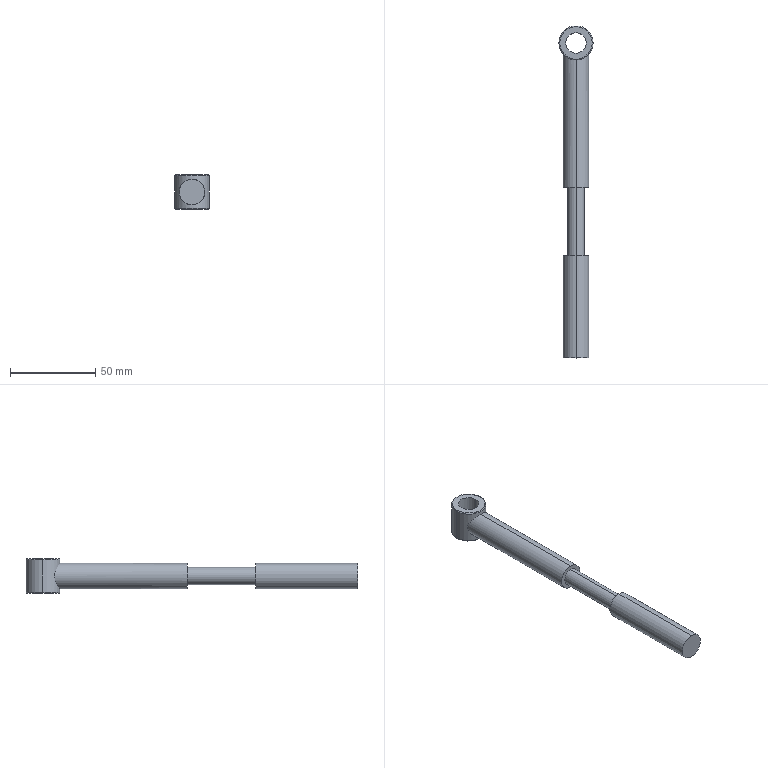Part | STEP file | piston rod | 1 solid | 19 faces | box 20 x 194.5 x 20 mm | volume 31059 mm3 | cylinder 10 | plane 5 | torus 4 | commonest cylinder face diameters 15 x4 10 x2 12 x2 20 x2
STEP:
#1=CARTESIAN_POINT('',(-10.,104.5,9.5));
#2=VERTEX_POINT('',#1);
#3=CARTESIAN_POINT('',(10.,104.5,9.5));
#4=VERTEX_POINT('',#3);
#5=CARTESIAN_POINT('',(0.,104.5,9.5));
#6=DIRECTION('',(0.,0.,-1.));
#7=DIRECTION('',(1.,0.,0.));
#8=AXIS2_PLACEMENT_3D('',#5,#6,#7);
#9=CIRCLE('',#8,10.);
#10=EDGE_CURVE('',#2,#4,#9,.T.);
#11=ORIENTED_EDGE('',*,*,#10,.F.);
#12=CARTESIAN_POINT('',(-9.5,104.5,10.));
#13=VERTEX_POINT('',#12);
#14=CARTESIAN_POINT('',(-9.5,104.5,9.5));
#15=DIRECTION('',(0.,1.,0.));
#16=DIRECTION('',(-1.,0.,0.));
#17=AXIS2_PLACEMENT_3D('',#14,#15,#16);
#18=CIRCLE('',#17,0.5);
#19=EDGE_CURVE('',#2,#13,#18,.T.);
#20=ORIENTED_EDGE('',*,*,#19,.T.);
#21=CARTESIAN_POINT('',(9.5,104.5,10.));
#22=VERTEX_POINT('',#21);
#23=CARTESIAN_POINT('',(0.,104.5,10.));
#24=DIRECTION('',(0.,0.,1.));
#25=DIRECTION('',(1.,0.,0.));
#26=AXIS2_PLACEMENT_3D('',#23,#24,#25);
#27=CIRCLE('',#26,9.5);
#28=EDGE_CURVE('',#22,#13,#27,.T.);
#29=ORIENTED_EDGE('',*,*,#28,.F.);
#30=CARTESIAN_POINT('',(9.5,104.5,9.5));
#31=DIRECTION('',(0.,-1.,0.));
#32=DIRECTION('',(0.,0.,-1.));
#33=AXIS2_PLACEMENT_3D('',#30,#31,#32);
#34=CIRCLE('',#33,0.5);
#35=EDGE_CURVE('',#4,#22,#34,.T.);
#36=ORIENTED_EDGE('',*,*,#35,.F.);
#37=EDGE_LOOP('',(#11,#20,#29,#36));
#38=FACE_OUTER_BOUND('',#37,.T.);
#39=CARTESIAN_POINT('',(0.,104.5,9.5));
#40=DIRECTION('',(0.,0.,1.));
#41=DIRECTION('',(1.,0.,0.));
#42=AXIS2_PLACEMENT_3D('',#39,#40,#41);
#43=TOROIDAL_SURFACE('',#42,9.5,0.5);
#44=ADVANCED_FACE('',(#38),#43,.T.);
#45=CARTESIAN_POINT('',(-9.5,104.5,-10.));
#46=VERTEX_POINT('',#45);
#47=CARTESIAN_POINT('',(9.5,104.5,-10.));
#48=VERTEX_POINT('',#47);
#49=CARTESIAN_POINT('',(0.,104.5,-10.));
#50=DIRECTION('',(0.,0.,-1.));
#51=DIRECTION('',(1.,0.,0.));
#52=AXIS2_PLACEMENT_3D('',#49,#50,#51);
#53=CIRCLE('',#52,9.5);
#54=EDGE_CURVE('',#46,#48,#53,.T.);
#55=ORIENTED_EDGE('',*,*,#54,.F.);
#56=CARTESIAN_POINT('',(-10.,104.5,-9.5));
#57=VERTEX_POINT('',#56);
#58=CARTESIAN_POINT('',(-9.5,104.5,-9.5));
#59=DIRECTION('',(0.,1.,0.));
#60=DIRECTION('',(-1.,0.,0.));
#61=AXIS2_PLACEMENT_3D('',#58,#59,#60);
#62=CIRCLE('',#61,0.5);
#63=EDGE_CURVE('',#46,#57,#62,.T.);
#64=ORIENTED_EDGE('',*,*,#63,.T.);
#65=CARTESIAN_POINT('',(10.,104.5,-9.5));
#66=VERTEX_POINT('',#65);
#67=CARTESIAN_POINT('',(0.,104.5,-9.5));
#68=DIRECTION('',(0.,0.,1.));
#69=DIRECTION('',(1.,0.,0.));
#70=AXIS2_PLACEMENT_3D('',#67,#68,#69);
#71=CIRCLE('',#70,10.);
#72=EDGE_CURVE('',#66,#57,#71,.T.);
#73=ORIENTED_EDGE('',*,*,#72,.F.);
#74=CARTESIAN_POINT('',(9.5,104.5,-9.5));
#75=DIRECTION('',(0.,-1.,0.));
#76=DIRECTION('',(0.,0.,-1.));
#77=AXIS2_PLACEMENT_3D('',#74,#75,#76);
#78=CIRCLE('',#77,0.5);
#79=EDGE_CURVE('',#48,#66,#78,.T.);
#80=ORIENTED_EDGE('',*,*,#79,.F.);
#81=EDGE_LOOP('',(#55,#64,#73,#80));
#82=FACE_OUTER_BOUND('',#81,.T.);
#83=CARTESIAN_POINT('',(0.,104.5,-9.5));
#84=DIRECTION('',(0.,0.,1.));
#85=DIRECTION('',(1.,0.,0.));
#86=AXIS2_PLACEMENT_3D('',#83,#84,#85);
#87=TOROIDAL_SURFACE('',#86,9.5,0.5);
#88=ADVANCED_FACE('',(#82),#87,.T.);
#89=CARTESIAN_POINT('',(-6.,104.5,-10.));
#90=VERTEX_POINT('',#89);
#91=CARTESIAN_POINT('',(6.,104.5,-10.));
#92=VERTEX_POINT('',#91);
#93=CARTESIAN_POINT('',(0.,104.5,-10.));
#94=DIRECTION('',(0.,0.,1.));
#95=DIRECTION('',(1.,0.,0.));
#96=AXIS2_PLACEMENT_3D('',#93,#94,#95);
#97=CIRCLE('',#96,6.);
#98=EDGE_CURVE('',#90,#92,#97,.T.);
#99=ORIENTED_EDGE('',*,*,#98,.F.);
#100=CARTESIAN_POINT('',(-6.,104.5,10.));
#101=VERTEX_POINT('',#100);
#102=CARTESIAN_POINT('',(-6.,104.5,-10.));
#103=DIRECTION('',(0.,0.,1.));
#104=VECTOR('',#103,1000.);
#105=LINE('',#102,#104);
#106=EDGE_CURVE('',#90,#101,#105,.T.);
#107=ORIENTED_EDGE('',*,*,#106,.T.);
#108=CARTESIAN_POINT('',(6.,104.5,10.));
#109=VERTEX_POINT('',#108);
#110=CARTESIAN_POINT('',(0.,104.5,10.));
#111=DIRECTION('',(0.,0.,1.));
#112=DIRECTION('',(1.,0.,0.));
#113=AXIS2_PLACEMENT_3D('',#110,#111,#112);
#114=CIRCLE('',#113,6.);
#115=EDGE_CURVE('',#101,#109,#114,.T.);
#116=ORIENTED_EDGE('',*,*,#115,.T.);
#117=CARTESIAN_POINT('',(6.,104.5,-10.));
#118=DIRECTION('',(0.,0.,1.));
#119=VECTOR('',#118,1000.);
#120=LINE('',#117,#119);
#121=EDGE_CURVE('',#92,#109,#120,.T.);
#122=ORIENTED_EDGE('',*,*,#121,.F.);
#123=EDGE_LOOP('',(#99,#107,#116,#122));
#124=FACE_OUTER_BOUND('',#123,.T.);
#125=CARTESIAN_POINT('',(0.,104.5,-10.));
#126=DIRECTION('',(0.,0.,1.));
#127=DIRECTION('',(1.,0.,0.));
#128=AXIS2_PLACEMENT_3D('',#125,#126,#127);
#129=CYLINDRICAL_SURFACE('',#128,6.);
#130=ADVANCED_FACE('',(#124),#129,.F.);
#131=ORIENTED_EDGE('',*,*,#10,.T.);
#132=CARTESIAN_POINT('',(10.,104.5,10.));
#133=DIRECTION('',(0.,0.,-1.));
#134=VECTOR('',#133,1000.);
#135=LINE('',#132,#134);
#136=EDGE_CURVE('',#4,#66,#135,.T.);
#137=ORIENTED_EDGE('',*,*,#136,.T.);
#138=ORIENTED_EDGE('',*,*,#72,.T.);
#139=CARTESIAN_POINT('',(-10.,104.5,10.));
#140=DIRECTION('',(0.,0.,-1.));
#141=VECTOR('',#140,1000.);
#142=LINE('',#139,#141);
#143=EDGE_CURVE('',#2,#57,#142,.T.);
#144=ORIENTED_EDGE('',*,*,#143,.F.);
#145=EDGE_LOOP('',(#131,#137,#138,#144));
#146=FACE_OUTER_BOUND('',#145,.T.);
#147=CARTESIAN_POINT('',(0.,104.5,10.));
#148=DIRECTION('',(0.,0.,-1.));
#149=DIRECTION('',(-1.,0.,0.));
#150=AXIS2_PLACEMENT_3D('',#147,#148,#149);
#151=CYLINDRICAL_SURFACE('',#150,10.);
#152=ADVANCED_FACE('',(#146),#151,.T.);
#153=CARTESIAN_POINT('',(0.,-20.,5.));
#154=VERTEX_POINT('',#153);
#155=CARTESIAN_POINT('',(0.,-20.,-5.));
#156=VERTEX_POINT('',#155);
#157=CARTESIAN_POINT('',(0.,-20.,0.));
#158=DIRECTION('',(0.,1.,0.));
#159=DIRECTION('',(0.,0.,1.));
#160=AXIS2_PLACEMENT_3D('',#157,#158,#159);
#161=CIRCLE('',#160,5.);
#162=EDGE_CURVE('',#154,#156,#161,.T.);
#163=ORIENTED_EDGE('',*,*,#162,.T.);
#164=CARTESIAN_POINT('',(0.,20.,-5.));
#165=VERTEX_POINT('',#164);
#166=CARTESIAN_POINT('',(0.,27.897,-5.));
#167=DIRECTION('',(0.,1.,0.));
#168=VECTOR('',#167,1000.);
#169=LINE('',#166,#168);
#170=EDGE_CURVE('',#156,#165,#169,.T.);
#171=ORIENTED_EDGE('',*,*,#170,.T.);
#172=CARTESIAN_POINT('',(0.,20.,5.));
#173=VERTEX_POINT('',#172);
#174=CARTESIAN_POINT('',(0.,20.,0.));
#175=DIRECTION('',(0.,1.,0.));
#176=DIRECTION('',(0.,0.,1.));
#177=AXIS2_PLACEMENT_3D('',#174,#175,#176);
#178=CIRCLE('',#177,5.);
#179=EDGE_CURVE('',#173,#165,#178,.T.);
#180=ORIENTED_EDGE('',*,*,#179,.F.);
#181=CARTESIAN_POINT('',(0.,27.897,5.));
#182=DIRECTION('',(0.,1.,0.));
#183=VECTOR('',#182,1000.);
#184=LINE('',#181,#183);
#185=EDGE_CURVE('',#154,#173,#184,.T.);
#186=ORIENTED_EDGE('',*,*,#185,.F.);
#187=EDGE_LOOP('',(#163,#171,#180,#186));
#188=FACE_OUTER_BOUND('',#187,.T.);
#189=CARTESIAN_POINT('',(0.,27.897,0.));
#190=DIRECTION('',(0.,1.,0.));
#191=DIRECTION('',(0.,0.,1.));
#192=AXIS2_PLACEMENT_3D('',#189,#190,#191);
#193=CYLINDRICAL_SURFACE('',#192,5.);
#194=ADVANCED_FACE('',(#188),#193,.T.);
#195=CARTESIAN_POINT('',(0.,20.,7.5));
#196=VERTEX_POINT('',#195);
#197=CARTESIAN_POINT('',(0.,20.,-7.5));
#198=VERTEX_POINT('',#197);
#199=CARTESIAN_POINT('',(0.,20.,0.));
#200=DIRECTION('',(0.,1.,0.));
#201=DIRECTION('',(0.,0.,1.));
#202=AXIS2_PLACEMENT_3D('',#199,#200,#201);
#203=CIRCLE('',#202,7.5);
#204=EDGE_CURVE('',#196,#198,#203,.T.);
#205=ORIENTED_EDGE('',*,*,#204,.T.);
#206=CARTESIAN_POINT('',(0.,94.5,-7.5));
#207=VERTEX_POINT('',#206);
#208=CARTESIAN_POINT('',(0.,63.204,-7.5));
#209=DIRECTION('',(0.,1.,0.));
#210=VECTOR('',#209,1000.);
#211=LINE('',#208,#210);
#212=EDGE_CURVE('',#198,#207,#211,.T.);
#213=ORIENTED_EDGE('',*,*,#212,.T.);
#214=CARTESIAN_POINT('',(0.,94.5,7.5));
#215=VERTEX_POINT('',#214);
#216=CARTESIAN_POINT('',(0.,94.5,-7.5));
#217=CARTESIAN_POINT('',(0.2563,94.5,-7.5));
#218=CARTESIAN_POINT('',(0.516,94.51,-7.487));
#219=CARTESIAN_POINT('',(1.029,94.55,-7.434));
#220=CARTESIAN_POINT('',(1.282,94.579,-7.394));
#221=CARTESIAN_POINT('',(1.778,94.656,-7.291));
#222=CARTESIAN_POINT('',(2.022,94.703,-7.227));
#223=CARTESIAN_POINT('',(2.502,94.815,-7.075));
#224=CARTESIAN_POINT('',(2.739,94.879,-6.986));
#225=CARTESIAN_POINT('',(3.422,95.092,-6.692));
#226=CARTESIAN_POINT('',(3.847,95.259,-6.457));
#227=CARTESIAN_POINT('',(4.643,95.632,-5.91));
#228=CARTESIAN_POINT('',(5.006,95.835,-5.604));
#229=CARTESIAN_POINT('',(5.501,96.147,-5.103));
#230=CARTESIAN_POINT('',(5.658,96.252,-4.929));
#231=CARTESIAN_POINT('',(5.955,96.465,-4.565));
#232=CARTESIAN_POINT('',(6.097,96.572,-4.375));
#233=CARTESIAN_POINT('',(6.489,96.884,-3.789));
#234=CARTESIAN_POINT('',(6.714,97.085,-3.376));
#235=CARTESIAN_POINT('',(6.995,97.353,-2.715));
#236=CARTESIAN_POINT('',(7.08,97.437,-2.487));
#237=CARTESIAN_POINT('',(7.228,97.589,-2.015));
#238=CARTESIAN_POINT('',(7.292,97.657,-1.772));
#239=CARTESIAN_POINT('',(7.394,97.767,-1.279));
#240=CARTESIAN_POINT('',(7.434,97.811,-1.029));
#241=CARTESIAN_POINT('',(7.486,97.87,-0.5188));
#242=CARTESIAN_POINT('',(7.5,97.886,-0.2571));
#243=CARTESIAN_POINT('',(7.5,97.886,0.2591));
#244=CARTESIAN_POINT('',(7.487,97.87,0.515));
#245=CARTESIAN_POINT('',(7.434,97.812,1.023));
#246=CARTESIAN_POINT('',(7.395,97.768,1.276));
#247=CARTESIAN_POINT('',(7.24,97.601,2.021));
#248=CARTESIAN_POINT('',(7.092,97.445,2.487));
#249=CARTESIAN_POINT('',(6.809,97.175,3.153));
#250=CARTESIAN_POINT('',(6.704,97.079,3.371));
#251=CARTESIAN_POINT('',(6.476,96.879,3.79));
#252=CARTESIAN_POINT('',(6.354,96.776,3.992));
#253=CARTESIAN_POINT('',(5.962,96.464,4.575));
#254=CARTESIAN_POINT('',(5.667,96.252,4.935));
#255=CARTESIAN_POINT('',(5.171,95.938,5.438));
#256=CARTESIAN_POINT('',(4.995,95.834,5.6));
#257=CARTESIAN_POINT('',(4.63,95.634,5.905));
#258=CARTESIAN_POINT('',(4.441,95.538,6.048));
#259=CARTESIAN_POINT('',(3.852,95.262,6.453));
#260=CARTESIAN_POINT('',(3.431,95.095,6.688));
#261=CARTESIAN_POINT('',(2.748,94.882,6.983));
#262=CARTESIAN_POINT('',(2.511,94.817,7.072));
#263=CARTESIAN_POINT('',(2.03,94.705,7.224));
#264=CARTESIAN_POINT('',(1.786,94.658,7.289));
#265=CARTESIAN_POINT('',(1.289,94.58,7.393));
#266=CARTESIAN_POINT('',(1.036,94.55,7.433));
#267=CARTESIAN_POINT('',(0.5214,94.51,7.486));
#268=CARTESIAN_POINT('',(0.2596,94.5,7.5));
#269=CARTESIAN_POINT('',(0.,94.5,7.5));
#270=B_SPLINE_CURVE_WITH_KNOTS('',3,(#216,#217,#218,#219,#220,#221,#222,#223,#224,#225,#226,#227,#228,#229,#230,#231,#232,#233,#234,#235,#236,#237,#238,#239,#240,#241,#242,#243,#244,#245,#246,#247,#248,#249,#250,#251,#252,#253,#254,#255,#256,#257,#258,#259,#260,#261,#262,#263,#264,#265,#266,#267,#268,#269),.UNSPECIFIED.,.F.,.F.,(4,2,2,2,2,2,2,2,2,2,2,2,2,2,2,2,2,2,2,2,2,2,2,2,2,2,4),(0.02456,0.02533,0.0261,0.02686,0.02763,0.02916,0.03069,0.03146,0.03222,0.03376,0.03452,0.03529,0.03605,0.03682,0.03759,0.03835,0.03989,0.04065,0.04142,0.04295,0.04372,0.04448,0.04601,0.04678,0.04755,0.04831,0.04908),.UNSPECIFIED.);
#271=EDGE_CURVE('',#207,#215,#270,.T.);
#272=ORIENTED_EDGE('',*,*,#271,.T.);
#273=CARTESIAN_POINT('',(0.,63.204,7.5));
#274=DIRECTION('',(0.,1.,0.));
#275=VECTOR('',#274,1000.);
#276=LINE('',#273,#275);
#277=EDGE_CURVE('',#196,#215,#276,.T.);
#278=ORIENTED_EDGE('',*,*,#277,.F.);
#279=EDGE_LOOP('',(#205,#213,#272,#278));
#280=FACE_OUTER_BOUND('',#279,.T.);
#281=CARTESIAN_POINT('',(0.,63.204,0.));
#282=DIRECTION('',(0.,1.,0.));
#283=DIRECTION('',(0.,0.,1.));
#284=AXIS2_PLACEMENT_3D('',#281,#282,#283);
#285=CYLINDRICAL_SURFACE('',#284,7.5);
#286=ADVANCED_FACE('',(#280),#285,.T.);
#287=CARTESIAN_POINT('',(0.,-80.,-7.5));
#288=VERTEX_POINT('',#287);
#289=CARTESIAN_POINT('',(0.,-80.,7.5));
#290=VERTEX_POINT('',#289);
#291=CARTESIAN_POINT('',(0.,-80.,0.));
#292=DIRECTION('',(0.,-1.,0.));
#293=DIRECTION('',(0.,0.,-1.));
#294=AXIS2_PLACEMENT_3D('',#291,#292,#293);
#295=CIRCLE('',#294,7.5);
#296=EDGE_CURVE('',#288,#290,#295,.T.);
#297=ORIENTED_EDGE('',*,*,#296,.F.);
#298=CARTESIAN_POINT('',(0.,-20.,-7.5));
#299=VERTEX_POINT('',#298);
#300=CARTESIAN_POINT('',(0.,63.204,-7.5));
#301=DIRECTION('',(0.,1.,0.));
#302=VECTOR('',#301,1000.);
#303=LINE('',#300,#302);
#304=EDGE_CURVE('',#288,#299,#303,.T.);
#305=ORIENTED_EDGE('',*,*,#304,.T.);
#306=CARTESIAN_POINT('',(0.,-20.,7.5));
#307=VERTEX_POINT('',#306);
#308=CARTESIAN_POINT('',(0.,-20.,0.));
#309=DIRECTION('',(0.,1.,0.));
#310=DIRECTION('',(0.,0.,1.));
#311=AXIS2_PLACEMENT_3D('',#308,#309,#310);
#312=CIRCLE('',#311,7.5);
#313=EDGE_CURVE('',#307,#299,#312,.T.);
#314=ORIENTED_EDGE('',*,*,#313,.F.);
#315=CARTESIAN_POINT('',(0.,63.204,7.5));
#316=DIRECTION('',(0.,1.,0.));
#317=VECTOR('',#316,1000.);
#318=LINE('',#315,#317);
#319=EDGE_CURVE('',#290,#307,#318,.T.);
#320=ORIENTED_EDGE('',*,*,#319,.F.);
#321=EDGE_LOOP('',(#297,#305,#314,#320));
#322=FACE_OUTER_BOUND('',#321,.T.);
#323=CARTESIAN_POINT('',(0.,63.204,0.));
#324=DIRECTION('',(0.,1.,0.));
#325=DIRECTION('',(0.,0.,1.));
#326=AXIS2_PLACEMENT_3D('',#323,#324,#325);
#327=CYLINDRICAL_SURFACE('',#326,7.5);
#328=ADVANCED_FACE('',(#322),#327,.T.);
#329=ORIENTED_EDGE('',*,*,#304,.F.);
#330=CARTESIAN_POINT('',(0.,-80.,0.));
#331=DIRECTION('',(0.,-1.,0.));
#332=DIRECTION('',(0.,0.,-1.));
#333=AXIS2_PLACEMENT_3D('',#330,#331,#332);
#334=CIRCLE('',#333,7.5);
#335=EDGE_CURVE('',#290,#288,#334,.T.);
#336=ORIENTED_EDGE('',*,*,#335,.F.);
#337=ORIENTED_EDGE('',*,*,#319,.T.);
#338=CARTESIAN_POINT('',(0.,-20.,0.));
#339=DIRECTION('',(0.,1.,0.));
#340=DIRECTION('',(0.,0.,1.));
#341=AXIS2_PLACEMENT_3D('',#338,#339,#340);
#342=CIRCLE('',#341,7.5);
#343=EDGE_CURVE('',#299,#307,#342,.T.);
#344=ORIENTED_EDGE('',*,*,#343,.F.);
#345=EDGE_LOOP('',(#329,#336,#337,#344));
#346=FACE_OUTER_BOUND('',#345,.T.);
#347=CARTESIAN_POINT('',(0.,63.204,0.));
#348=DIRECTION('',(0.,1.,0.));
#349=DIRECTION('',(0.,0.,1.));
#350=AXIS2_PLACEMENT_3D('',#347,#348,#349);
#351=CYLINDRICAL_SURFACE('',#350,7.5);
#352=ADVANCED_FACE('',(#346),#351,.T.);
#353=ORIENTED_EDGE('',*,*,#212,.F.);
#354=CARTESIAN_POINT('',(0.,20.,0.));
#355=DIRECTION('',(0.,1.,0.));
#356=DIRECTION('',(0.,0.,1.));
#357=AXIS2_PLACEMENT_3D('',#354,#355,#356);
#358=CIRCLE('',#357,7.5);
#359=EDGE_CURVE('',#198,#196,#358,.T.);
#360=ORIENTED_EDGE('',*,*,#359,.T.);
#361=ORIENTED_EDGE('',*,*,#277,.T.);
#362=CARTESIAN_POINT('',(0.,94.5,7.5));
#363=CARTESIAN_POINT('',(-0.5202,94.5,7.5));
#364=CARTESIAN_POINT('',(-1.028,94.54,7.446));
#365=CARTESIAN_POINT('',(-1.773,94.655,7.292));
#366=CARTESIAN_POINT('',(-2.02,94.703,7.227));
#367=CARTESIAN_POINT('',(-2.503,94.815,7.075));
#368=CARTESIAN_POINT('',(-2.736,94.879,6.987));
#369=CARTESIAN_POINT('',(-3.19,95.019,6.792));
#370=CARTESIAN_POINT('',(-3.41,95.097,6.685));
#371=CARTESIAN_POINT('',(-3.837,95.262,6.449));
#372=CARTESIAN_POINT('',(-4.044,95.352,6.321));
#373=CARTESIAN_POINT('',(-4.641,95.631,5.911));
#374=CARTESIAN_POINT('',(-5.003,95.833,5.607));
#375=CARTESIAN_POINT('',(-5.665,96.25,4.938));
#376=CARTESIAN_POINT('',(-5.965,96.467,4.571));
#377=CARTESIAN_POINT('',(-6.487,96.882,3.793));
#378=CARTESIAN_POINT('',(-6.713,97.083,3.38));
#379=CARTESIAN_POINT('',(-6.996,97.354,2.714));
#380=CARTESIAN_POINT('',(-7.082,97.439,2.482));
#381=CARTESIAN_POINT('',(-7.23,97.59,2.011));
#382=CARTESIAN_POINT('',(-7.292,97.657,1.771));
#383=CARTESIAN_POINT('',(-7.394,97.767,1.279));
#384=CARTESIAN_POINT('',(-7.434,97.811,1.027));
#385=CARTESIAN_POINT('',(-7.487,97.871,0.5128));
#386=CARTESIAN_POINT('',(-7.5,97.886,0.2562));
#387=CARTESIAN_POINT('',(-7.5,97.886,-0.256));
#388=CARTESIAN_POINT('',(-7.487,97.871,-0.5115));
#389=CARTESIAN_POINT('',(-7.435,97.812,-1.021));
#390=CARTESIAN_POINT('',(-7.395,97.768,-1.277));
#391=CARTESIAN_POINT('',(-7.292,97.657,-1.771));
#392=CARTESIAN_POINT('',(-7.229,97.59,-2.011));
#393=CARTESIAN_POINT('',(-7.082,97.439,-2.482));
#394=CARTESIAN_POINT('',(-6.996,97.353,-2.714));
#395=CARTESIAN_POINT('',(-6.712,97.082,-3.382));
#396=CARTESIAN_POINT('',(-6.485,96.881,-3.796));
#397=CARTESIAN_POINT('',(-5.962,96.465,-4.574));
#398=CARTESIAN_POINT('',(-5.661,96.247,-4.942));
#399=CARTESIAN_POINT('',(-5.,95.831,-5.61));
#400=CARTESIAN_POINT('',(-4.639,95.63,-5.913));
#401=CARTESIAN_POINT('',(-3.848,95.26,-6.455));
#402=CARTESIAN_POINT('',(-3.415,95.089,-6.696));
#403=CARTESIAN_POINT('',(-2.734,94.878,-6.988));
#404=CARTESIAN_POINT('',(-2.501,94.815,-7.075));
#405=CARTESIAN_POINT('',(-2.022,94.704,-7.227));
#406=CARTESIAN_POINT('',(-1.775,94.655,-7.292));
#407=CARTESIAN_POINT('',(-1.022,94.539,-7.448));
#408=CARTESIAN_POINT('',(-0.5138,94.5,-7.5));
#409=CARTESIAN_POINT('',(0.,94.5,-7.5));
#410=B_SPLINE_CURVE_WITH_KNOTS('',3,(#362,#363,#364,#365,#366,#367,#368,#369,#370,#371,#372,#373,#374,#375,#376,#377,#378,#379,#380,#381,#382,#383,#384,#385,#386,#387,#388,#389,#390,#391,#392,#393,#394,#395,#396,#397,#398,#399,#400,#401,#402,#403,#404,#405,#406,#407,#408,#409),.UNSPECIFIED.,.F.,.F.,(4,2,2,2,2,2,2,2,2,2,2,2,2,2,2,2,2,2,2,2,2,2,2,4),(0.,0.001535,0.002303,0.003071,0.003838,0.004606,0.006141,0.007676,0.009212,0.009979,0.01075,0.01151,0.01228,0.01305,0.01382,0.01459,0.01535,0.01689,0.01842,0.01996,0.02149,0.02226,0.02303,0.02456),.UNSPECIFIED.);
#411=EDGE_CURVE('',#215,#207,#410,.T.);
#412=ORIENTED_EDGE('',*,*,#411,.T.);
#413=EDGE_LOOP('',(#353,#360,#361,#412));
#414=FACE_OUTER_BOUND('',#413,.T.);
#415=CARTESIAN_POINT('',(0.,63.204,0.));
#416=DIRECTION('',(0.,1.,0.));
#417=DIRECTION('',(0.,0.,1.));
#418=AXIS2_PLACEMENT_3D('',#415,#416,#417);
#419=CYLINDRICAL_SURFACE('',#418,7.5);
#420=ADVANCED_FACE('',(#414),#419,.T.);
#421=ORIENTED_EDGE('',*,*,#204,.F.);
#422=ORIENTED_EDGE('',*,*,#359,.F.);
#423=EDGE_LOOP('',(#421,#422));
#424=FACE_OUTER_BOUND('',#423,.T.);
#425=ORIENTED_EDGE('',*,*,#179,.T.);
#426=CARTESIAN_POINT('',(0.,20.,0.));
#427=DIRECTION('',(0.,1.,0.));
#428=DIRECTION('',(0.,0.,1.));
#429=AXIS2_PLACEMENT_3D('',#426,#427,#428);
#430=CIRCLE('',#429,5.);
#431=EDGE_CURVE('',#165,#173,#430,.T.);
#432=ORIENTED_EDGE('',*,*,#431,.T.);
#433=EDGE_LOOP('',(#425,#432));
#434=FACE_BOUND('',#433,.T.);
#435=CARTESIAN_POINT('',(-5.,20.,0.));
#436=DIRECTION('',(0.,1.,0.));
#437=DIRECTION('',(0.,0.,1.));
#438=AXIS2_PLACEMENT_3D('',#435,#436,#437);
#439=PLANE('',#438);
#440=ADVANCED_FACE('',(#424,#434),#439,.F.);
#441=ORIENTED_EDGE('',*,*,#170,.F.);
#442=CARTESIAN_POINT('',(0.,-20.,0.));
#443=DIRECTION('',(0.,1.,0.));
#444=DIRECTION('',(0.,0.,1.));
#445=AXIS2_PLACEMENT_3D('',#442,#443,#444);
#446=CIRCLE('',#445,5.);
#447=EDGE_CURVE('',#156,#154,#446,.T.);
#448=ORIENTED_EDGE('',*,*,#447,.T.);
#449=ORIENTED_EDGE('',*,*,#185,.T.);
#450=ORIENTED_EDGE('',*,*,#431,.F.);
#451=EDGE_LOOP('',(#441,#448,#449,#450));
#452=FACE_OUTER_BOUND('',#451,.T.);
#453=CARTESIAN_POINT('',(0.,27.897,0.));
#454=DIRECTION('',(0.,1.,0.));
#455=DIRECTION('',(0.,0.,1.));
#456=AXIS2_PLACEMENT_3D('',#453,#454,#455);
#457=CYLINDRICAL_SURFACE('',#456,5.);
#458=ADVANCED_FACE('',(#452),#457,.T.);
#459=ORIENTED_EDGE('',*,*,#162,.F.);
#460=ORIENTED_EDGE('',*,*,#447,.F.);
#461=EDGE_LOOP('',(#459,#460));
#462=FACE_BOUND('',#461,.T.);
#463=ORIENTED_EDGE('',*,*,#313,.T.);
#464=ORIENTED_EDGE('',*,*,#343,.T.);
#465=EDGE_LOOP('',(#463,#464));
#466=FACE_OUTER_BOUND('',#465,.T.);
#467=CARTESIAN_POINT('',(-5.,-20.,0.));
#468=DIRECTION('',(0.,-1.,0.));
#469=DIRECTION('',(0.,0.,-1.));
#470=AXIS2_PLACEMENT_3D('',#467,#468,#469);
#471=PLANE('',#470);
#472=ADVANCED_FACE('',(#462,#466),#471,.F.);
#473=ORIENTED_EDGE('',*,*,#136,.F.);
#474=CARTESIAN_POINT('',(0.,104.5,9.5));
#475=DIRECTION('',(0.,0.,-1.));
#476=DIRECTION('',(1.,0.,0.));
#477=AXIS2_PLACEMENT_3D('',#474,#475,#476);
#478=CIRCLE('',#477,10.);
#479=EDGE_CURVE('',#4,#2,#478,.T.);
#480=ORIENTED_EDGE('',*,*,#479,.T.);
#481=ORIENTED_EDGE('',*,*,#143,.T.);
#482=CARTESIAN_POINT('',(0.,104.5,-9.5));
#483=DIRECTION('',(0.,0.,1.));
#484=DIRECTION('',(1.,0.,0.));
#485=AXIS2_PLACEMENT_3D('',#482,#483,#484);
#486=CIRCLE('',#485,10.);
#487=EDGE_CURVE('',#57,#66,#486,.T.);
#488=ORIENTED_EDGE('',*,*,#487,.T.);
#489=EDGE_LOOP('',(#473,#480,#481,#488));
#490=FACE_OUTER_BOUND('',#489,.T.);
#491=ORIENTED_EDGE('',*,*,#411,.F.);
#492=ORIENTED_EDGE('',*,*,#271,.F.);
#493=EDGE_LOOP('',(#491,#492));
#494=FACE_BOUND('',#493,.T.);
#495=CARTESIAN_POINT('',(0.,104.5,10.));
#496=DIRECTION('',(0.,0.,-1.));
#497=DIRECTION('',(-1.,0.,0.));
#498=AXIS2_PLACEMENT_3D('',#495,#496,#497);
#499=CYLINDRICAL_SURFACE('',#498,10.);
#500=ADVANCED_FACE('',(#490,#494),#499,.T.);
#501=ORIENTED_EDGE('',*,*,#28,.T.);
#502=CARTESIAN_POINT('',(0.,104.5,10.));
#503=DIRECTION('',(0.,0.,1.));
#504=DIRECTION('',(1.,0.,0.));
#505=AXIS2_PLACEMENT_3D('',#502,#503,#504);
#506=CIRCLE('',#505,9.5);
#507=EDGE_CURVE('',#13,#22,#506,.T.);
#508=ORIENTED_EDGE('',*,*,#507,.T.);
#509=EDGE_LOOP('',(#501,#508));
#510=FACE_OUTER_BOUND('',#509,.T.);
#511=CARTESIAN_POINT('',(0.,104.5,10.));
#512=DIRECTION('',(0.,0.,1.));
#513=DIRECTION('',(1.,0.,0.));
#514=AXIS2_PLACEMENT_3D('',#511,#512,#513);
#515=CIRCLE('',#514,6.);
#516=EDGE_CURVE('',#109,#101,#515,.T.);
#517=ORIENTED_EDGE('',*,*,#516,.F.);
#518=ORIENTED_EDGE('',*,*,#115,.F.);
#519=EDGE_LOOP('',(#517,#518));
#520=FACE_BOUND('',#519,.T.);
#521=CARTESIAN_POINT('',(0.,104.5,10.));
#522=DIRECTION('',(0.,0.,1.));
#523=DIRECTION('',(1.,0.,0.));
#524=AXIS2_PLACEMENT_3D('',#521,#522,#523);
#525=PLANE('',#524);
#526=ADVANCED_FACE('',(#510,#520),#525,.T.);
#527=CARTESIAN_POINT('',(0.,104.5,-10.));
#528=DIRECTION('',(0.,0.,-1.));
#529=DIRECTION('',(1.,0.,0.));
#530=AXIS2_PLACEMENT_3D('',#527,#528,#529);
#531=CIRCLE('',#530,9.5);
#532=EDGE_CURVE('',#48,#46,#531,.T.);
#533=ORIENTED_EDGE('',*,*,#532,.T.);
#534=ORIENTED_EDGE('',*,*,#54,.T.);
#535=EDGE_LOOP('',(#533,#534));
#536=FACE_OUTER_BOUND('',#535,.T.);
#537=CARTESIAN_POINT('',(0.,104.5,-10.));
#538=DIRECTION('',(0.,0.,1.));
#539=DIRECTION('',(1.,0.,0.));
#540=AXIS2_PLACEMENT_3D('',#537,#538,#539);
#541=CIRCLE('',#540,6.);
#542=EDGE_CURVE('',#92,#90,#541,.T.);
#543=ORIENTED_EDGE('',*,*,#542,.T.);
#544=ORIENTED_EDGE('',*,*,#98,.T.);
#545=EDGE_LOOP('',(#543,#544));
#546=FACE_BOUND('',#545,.T.);
#547=CARTESIAN_POINT('',(0.,104.5,-10.));
#548=DIRECTION('',(0.,0.,1.));
#549=DIRECTION('',(1.,0.,0.));
#550=AXIS2_PLACEMENT_3D('',#547,#548,#549);
#551=PLANE('',#550);
#552=ADVANCED_FACE('',(#536,#546),#551,.F.);
#553=ORIENTED_EDGE('',*,*,#106,.F.);
#554=ORIENTED_EDGE('',*,*,#542,.F.);
#555=ORIENTED_EDGE('',*,*,#121,.T.);
#556=ORIENTED_EDGE('',*,*,#516,.T.);
#557=EDGE_LOOP('',(#553,#554,#555,#556));
#558=FACE_OUTER_BOUND('',#557,.T.);
#559=CARTESIAN_POINT('',(0.,104.5,-10.));
#560=DIRECTION('',(0.,0.,1.));
#561=DIRECTION('',(1.,0.,0.));
#562=AXIS2_PLACEMENT_3D('',#559,#560,#561);
#563=CYLINDRICAL_SURFACE('',#562,6.);
#564=ADVANCED_FACE('',(#558),#563,.F.);
#565=ORIENTED_EDGE('',*,*,#63,.F.);
#566=ORIENTED_EDGE('',*,*,#532,.F.);
#567=ORIENTED_EDGE('',*,*,#79,.T.);
#568=ORIENTED_EDGE('',*,*,#487,.F.);
#569=EDGE_LOOP('',(#565,#566,#567,#568));
#570=FACE_OUTER_BOUND('',#569,.T.);
#571=CARTESIAN_POINT('',(0.,104.5,-9.5));
#572=DIRECTION('',(0.,0.,1.));
#573=DIRECTION('',(1.,0.,0.));
#574=AXIS2_PLACEMENT_3D('',#571,#572,#573);
#575=TOROIDAL_SURFACE('',#574,9.5,0.5);
#576=ADVANCED_FACE('',(#570),#575,.T.);
#577=ORIENTED_EDGE('',*,*,#19,.F.);
#578=ORIENTED_EDGE('',*,*,#479,.F.);
#579=ORIENTED_EDGE('',*,*,#35,.T.);
#580=ORIENTED_EDGE('',*,*,#507,.F.);
#581=EDGE_LOOP('',(#577,#578,#579,#580));
#582=FACE_OUTER_BOUND('',#581,.T.);
#583=CARTESIAN_POINT('',(0.,104.5,9.5));
#584=DIRECTION('',(0.,0.,1.));
#585=DIRECTION('',(1.,0.,0.));
#586=AXIS2_PLACEMENT_3D('',#583,#584,#585);
#587=TOROIDAL_SURFACE('',#586,9.5,0.5);
#588=ADVANCED_FACE('',(#582),#587,.T.);
#589=ORIENTED_EDGE('',*,*,#335,.T.);
#590=ORIENTED_EDGE('',*,*,#296,.T.);
#591=EDGE_LOOP('',(#589,#590));
#592=FACE_OUTER_BOUND('',#591,.T.);
#593=CARTESIAN_POINT('',(0.,-80.,0.));
#594=DIRECTION('',(0.,-1.,0.));
#595=DIRECTION('',(0.,0.,-1.));
#596=AXIS2_PLACEMENT_3D('',#593,#594,#595);
#597=PLANE('',#596);
#598=ADVANCED_FACE('',(#592),#597,.T.);
#599=CLOSED_SHELL('',(#44,#88,#130,#152,#194,#286,#328,#352,#420,#440,#458,#472,#500,#526,#552,#564,#576,#588,#598));
#600=MANIFOLD_SOLID_BREP('',#599);
#601=CARTESIAN_POINT('',(0.,0.,0.));
#602=DIRECTION('',(0.,0.,1.));
#603=DIRECTION('',(1.,0.,0.));
#604=AXIS2_PLACEMENT_3D('',#601,#602,#603);
#605=(LENGTH_UNIT()NAMED_UNIT(*)SI_UNIT(.MILLI.,.METRE.));
#606=UNCERTAINTY_MEASURE_WITH_UNIT(LENGTH_MEASURE(0.00001),#605,'','');
#607=(NAMED_UNIT(*)PLANE_ANGLE_UNIT()SI_UNIT($,.RADIAN.));
#608=(NAMED_UNIT(*)SI_UNIT($,.STERADIAN.)SOLID_ANGLE_UNIT());
#609=(GEOMETRIC_REPRESENTATION_CONTEXT(3)GLOBAL_UNCERTAINTY_ASSIGNED_CONTEXT((#606))GLOBAL_UNIT_ASSIGNED_CONTEXT((#605,#607,#608))REPRESENTATION_CONTEXT('',''));
#610=ADVANCED_BREP_SHAPE_REPRESENTATION('',(#600,#604),#609);